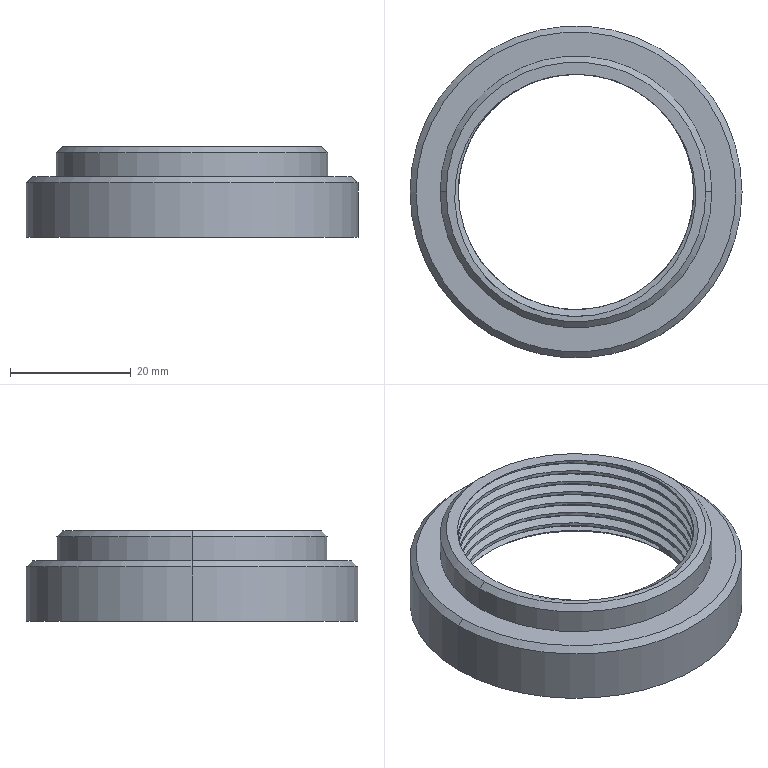Part | SolidWorks | features Chamfer 1, Extrusion 1, ICE 1, SweepThread 1 | 1 solid | 32 faces | box 55 x 55 x 15 mm | volume 12694 mm3 | cylinder 19 | cone 6 | plane 4 | spline 3 | commonest cylinder face diameters 39 x15 45 x2 55 x2